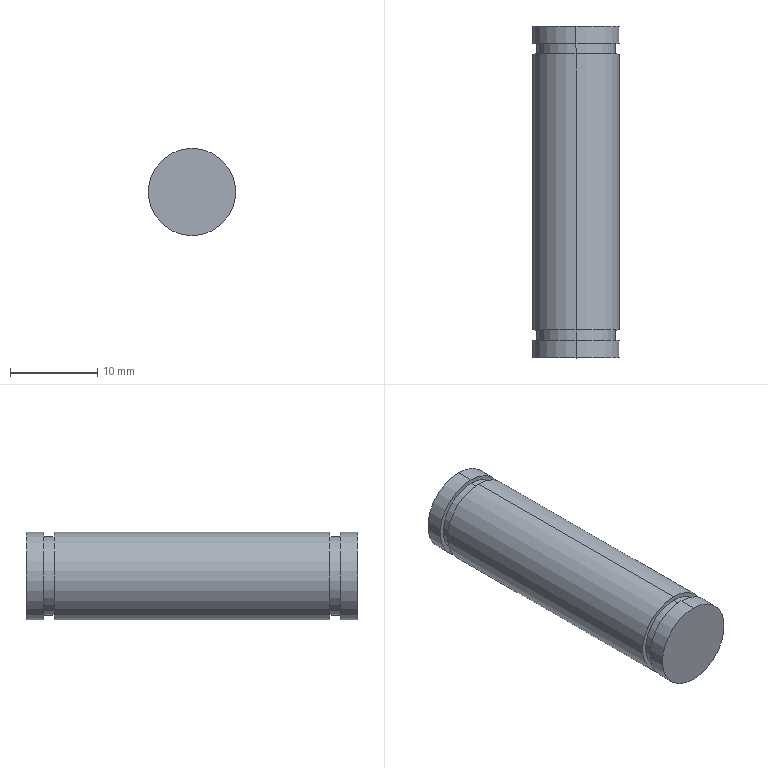Part | SolidWorks | features Revolution 1 | 1 solid | 16 faces | box 10 x 38 x 10 mm | volume 2949 mm3 | cylinder 10 | plane 6 | commonest cylinder face diameters 10 x6 9 x4
STEP:
#1=CARTESIAN_POINT('',(0.,-17.,4.5));
#2=VERTEX_POINT('',#1);
#3=CARTESIAN_POINT('',(0.,-17.,-4.5));
#4=VERTEX_POINT('',#3);
#5=CARTESIAN_POINT('',(0.,-17.,0.));
#6=DIRECTION('',(0.,1.,0.));
#7=DIRECTION('',(0.,0.,1.));
#8=AXIS2_PLACEMENT_3D('',#5,#6,#7);
#9=CIRCLE('',#8,4.5);
#10=EDGE_CURVE('',#2,#4,#9,.T.);
#11=ORIENTED_EDGE('',*,*,#10,.T.);
#12=CARTESIAN_POINT('',(0.,-15.8,-4.5));
#13=VERTEX_POINT('',#12);
#14=CARTESIAN_POINT('',(0.,-19.,-4.5));
#15=DIRECTION('',(0.,1.,0.));
#16=VECTOR('',#15,1000.);
#17=LINE('',#14,#16);
#18=EDGE_CURVE('',#4,#13,#17,.T.);
#19=ORIENTED_EDGE('',*,*,#18,.T.);
#20=CARTESIAN_POINT('',(0.,-15.8,4.5));
#21=VERTEX_POINT('',#20);
#22=CARTESIAN_POINT('',(0.,-15.8,0.));
#23=DIRECTION('',(0.,1.,0.));
#24=DIRECTION('',(0.,0.,1.));
#25=AXIS2_PLACEMENT_3D('',#22,#23,#24);
#26=CIRCLE('',#25,4.5);
#27=EDGE_CURVE('',#21,#13,#26,.T.);
#28=ORIENTED_EDGE('',*,*,#27,.F.);
#29=CARTESIAN_POINT('',(0.,-19.,4.5));
#30=DIRECTION('',(0.,1.,0.));
#31=VECTOR('',#30,1000.);
#32=LINE('',#29,#31);
#33=EDGE_CURVE('',#2,#21,#32,.T.);
#34=ORIENTED_EDGE('',*,*,#33,.F.);
#35=EDGE_LOOP('',(#11,#19,#28,#34));
#36=FACE_OUTER_BOUND('',#35,.T.);
#37=CARTESIAN_POINT('',(0.,-19.,0.));
#38=DIRECTION('',(0.,1.,0.));
#39=DIRECTION('',(0.,0.,1.));
#40=AXIS2_PLACEMENT_3D('',#37,#38,#39);
#41=CYLINDRICAL_SURFACE('',#40,4.5);
#42=ADVANCED_FACE('',(#36),#41,.T.);
#43=CARTESIAN_POINT('',(0.,-15.8,5.));
#44=VERTEX_POINT('',#43);
#45=CARTESIAN_POINT('',(0.,-15.8,-5.));
#46=VERTEX_POINT('',#45);
#47=CARTESIAN_POINT('',(0.,-15.8,0.));
#48=DIRECTION('',(0.,1.,0.));
#49=DIRECTION('',(0.,0.,1.));
#50=AXIS2_PLACEMENT_3D('',#47,#48,#49);
#51=CIRCLE('',#50,5.);
#52=EDGE_CURVE('',#44,#46,#51,.T.);
#53=ORIENTED_EDGE('',*,*,#52,.T.);
#54=CARTESIAN_POINT('',(0.,15.8,-5.));
#55=VERTEX_POINT('',#54);
#56=CARTESIAN_POINT('',(0.,-19.,-5.));
#57=DIRECTION('',(0.,1.,0.));
#58=VECTOR('',#57,1000.);
#59=LINE('',#56,#58);
#60=EDGE_CURVE('',#46,#55,#59,.T.);
#61=ORIENTED_EDGE('',*,*,#60,.T.);
#62=CARTESIAN_POINT('',(0.,15.8,5.));
#63=VERTEX_POINT('',#62);
#64=CARTESIAN_POINT('',(0.,15.8,0.));
#65=DIRECTION('',(0.,1.,0.));
#66=DIRECTION('',(0.,0.,1.));
#67=AXIS2_PLACEMENT_3D('',#64,#65,#66);
#68=CIRCLE('',#67,5.);
#69=EDGE_CURVE('',#63,#55,#68,.T.);
#70=ORIENTED_EDGE('',*,*,#69,.F.);
#71=CARTESIAN_POINT('',(0.,-19.,5.));
#72=DIRECTION('',(0.,1.,0.));
#73=VECTOR('',#72,1000.);
#74=LINE('',#71,#73);
#75=EDGE_CURVE('',#44,#63,#74,.T.);
#76=ORIENTED_EDGE('',*,*,#75,.F.);
#77=EDGE_LOOP('',(#53,#61,#70,#76));
#78=FACE_OUTER_BOUND('',#77,.T.);
#79=CARTESIAN_POINT('',(0.,-19.,0.));
#80=DIRECTION('',(0.,1.,0.));
#81=DIRECTION('',(0.,0.,1.));
#82=AXIS2_PLACEMENT_3D('',#79,#80,#81);
#83=CYLINDRICAL_SURFACE('',#82,5.);
#84=ADVANCED_FACE('',(#78),#83,.T.);
#85=CARTESIAN_POINT('',(0.,15.8,4.5));
#86=VERTEX_POINT('',#85);
#87=CARTESIAN_POINT('',(0.,15.8,-4.5));
#88=VERTEX_POINT('',#87);
#89=CARTESIAN_POINT('',(0.,15.8,0.));
#90=DIRECTION('',(0.,1.,0.));
#91=DIRECTION('',(0.,0.,1.));
#92=AXIS2_PLACEMENT_3D('',#89,#90,#91);
#93=CIRCLE('',#92,4.5);
#94=EDGE_CURVE('',#86,#88,#93,.T.);
#95=ORIENTED_EDGE('',*,*,#94,.T.);
#96=CARTESIAN_POINT('',(0.,17.,-4.5));
#97=VERTEX_POINT('',#96);
#98=CARTESIAN_POINT('',(0.,-19.,-4.5));
#99=DIRECTION('',(0.,1.,0.));
#100=VECTOR('',#99,1000.);
#101=LINE('',#98,#100);
#102=EDGE_CURVE('',#88,#97,#101,.T.);
#103=ORIENTED_EDGE('',*,*,#102,.T.);
#104=CARTESIAN_POINT('',(0.,17.,4.5));
#105=VERTEX_POINT('',#104);
#106=CARTESIAN_POINT('',(0.,17.,0.));
#107=DIRECTION('',(0.,1.,0.));
#108=DIRECTION('',(0.,0.,1.));
#109=AXIS2_PLACEMENT_3D('',#106,#107,#108);
#110=CIRCLE('',#109,4.5);
#111=EDGE_CURVE('',#105,#97,#110,.T.);
#112=ORIENTED_EDGE('',*,*,#111,.F.);
#113=CARTESIAN_POINT('',(0.,-19.,4.5));
#114=DIRECTION('',(0.,1.,0.));
#115=VECTOR('',#114,1000.);
#116=LINE('',#113,#115);
#117=EDGE_CURVE('',#86,#105,#116,.T.);
#118=ORIENTED_EDGE('',*,*,#117,.F.);
#119=EDGE_LOOP('',(#95,#103,#112,#118));
#120=FACE_OUTER_BOUND('',#119,.T.);
#121=CARTESIAN_POINT('',(0.,-19.,0.));
#122=DIRECTION('',(0.,1.,0.));
#123=DIRECTION('',(0.,0.,1.));
#124=AXIS2_PLACEMENT_3D('',#121,#122,#123);
#125=CYLINDRICAL_SURFACE('',#124,4.5);
#126=ADVANCED_FACE('',(#120),#125,.T.);
#127=CARTESIAN_POINT('',(0.,17.,5.));
#128=VERTEX_POINT('',#127);
#129=CARTESIAN_POINT('',(0.,17.,-5.));
#130=VERTEX_POINT('',#129);
#131=CARTESIAN_POINT('',(0.,17.,0.));
#132=DIRECTION('',(0.,1.,0.));
#133=DIRECTION('',(0.,0.,1.));
#134=AXIS2_PLACEMENT_3D('',#131,#132,#133);
#135=CIRCLE('',#134,5.);
#136=EDGE_CURVE('',#128,#130,#135,.T.);
#137=ORIENTED_EDGE('',*,*,#136,.T.);
#138=CARTESIAN_POINT('',(0.,19.,-5.));
#139=VERTEX_POINT('',#138);
#140=CARTESIAN_POINT('',(0.,-19.,-5.));
#141=DIRECTION('',(0.,1.,0.));
#142=VECTOR('',#141,1000.);
#143=LINE('',#140,#142);
#144=EDGE_CURVE('',#130,#139,#143,.T.);
#145=ORIENTED_EDGE('',*,*,#144,.T.);
#146=CARTESIAN_POINT('',(0.,19.,5.));
#147=VERTEX_POINT('',#146);
#148=CARTESIAN_POINT('',(0.,19.,0.));
#149=DIRECTION('',(0.,1.,0.));
#150=DIRECTION('',(0.,0.,1.));
#151=AXIS2_PLACEMENT_3D('',#148,#149,#150);
#152=CIRCLE('',#151,5.);
#153=EDGE_CURVE('',#147,#139,#152,.T.);
#154=ORIENTED_EDGE('',*,*,#153,.F.);
#155=CARTESIAN_POINT('',(0.,-19.,5.));
#156=DIRECTION('',(0.,1.,0.));
#157=VECTOR('',#156,1000.);
#158=LINE('',#155,#157);
#159=EDGE_CURVE('',#128,#147,#158,.T.);
#160=ORIENTED_EDGE('',*,*,#159,.F.);
#161=EDGE_LOOP('',(#137,#145,#154,#160));
#162=FACE_OUTER_BOUND('',#161,.T.);
#163=CARTESIAN_POINT('',(0.,-19.,0.));
#164=DIRECTION('',(0.,1.,0.));
#165=DIRECTION('',(0.,0.,1.));
#166=AXIS2_PLACEMENT_3D('',#163,#164,#165);
#167=CYLINDRICAL_SURFACE('',#166,5.);
#168=ADVANCED_FACE('',(#162),#167,.T.);
#169=CARTESIAN_POINT('',(0.,-19.,5.));
#170=VERTEX_POINT('',#169);
#171=CARTESIAN_POINT('',(0.,-19.,-5.));
#172=VERTEX_POINT('',#171);
#173=CARTESIAN_POINT('',(0.,-19.,0.));
#174=DIRECTION('',(0.,1.,0.));
#175=DIRECTION('',(0.,0.,1.));
#176=AXIS2_PLACEMENT_3D('',#173,#174,#175);
#177=CIRCLE('',#176,5.);
#178=EDGE_CURVE('',#170,#172,#177,.T.);
#179=ORIENTED_EDGE('',*,*,#178,.T.);
#180=CARTESIAN_POINT('',(0.,-17.,-5.));
#181=VERTEX_POINT('',#180);
#182=CARTESIAN_POINT('',(0.,-19.,-5.));
#183=DIRECTION('',(0.,1.,0.));
#184=VECTOR('',#183,1000.);
#185=LINE('',#182,#184);
#186=EDGE_CURVE('',#172,#181,#185,.T.);
#187=ORIENTED_EDGE('',*,*,#186,.T.);
#188=CARTESIAN_POINT('',(0.,-17.,5.));
#189=VERTEX_POINT('',#188);
#190=CARTESIAN_POINT('',(0.,-17.,0.));
#191=DIRECTION('',(0.,1.,0.));
#192=DIRECTION('',(0.,0.,1.));
#193=AXIS2_PLACEMENT_3D('',#190,#191,#192);
#194=CIRCLE('',#193,5.);
#195=EDGE_CURVE('',#189,#181,#194,.T.);
#196=ORIENTED_EDGE('',*,*,#195,.F.);
#197=CARTESIAN_POINT('',(0.,-19.,5.));
#198=DIRECTION('',(0.,1.,0.));
#199=VECTOR('',#198,1000.);
#200=LINE('',#197,#199);
#201=EDGE_CURVE('',#170,#189,#200,.T.);
#202=ORIENTED_EDGE('',*,*,#201,.F.);
#203=EDGE_LOOP('',(#179,#187,#196,#202));
#204=FACE_OUTER_BOUND('',#203,.T.);
#205=CARTESIAN_POINT('',(0.,-19.,0.));
#206=DIRECTION('',(0.,1.,0.));
#207=DIRECTION('',(0.,0.,1.));
#208=AXIS2_PLACEMENT_3D('',#205,#206,#207);
#209=CYLINDRICAL_SURFACE('',#208,5.);
#210=ADVANCED_FACE('',(#204),#209,.T.);
#211=ORIENTED_EDGE('',*,*,#186,.F.);
#212=CARTESIAN_POINT('',(0.,-19.,0.));
#213=DIRECTION('',(0.,1.,0.));
#214=DIRECTION('',(0.,0.,1.));
#215=AXIS2_PLACEMENT_3D('',#212,#213,#214);
#216=CIRCLE('',#215,5.);
#217=EDGE_CURVE('',#172,#170,#216,.T.);
#218=ORIENTED_EDGE('',*,*,#217,.T.);
#219=ORIENTED_EDGE('',*,*,#201,.T.);
#220=CARTESIAN_POINT('',(0.,-17.,0.));
#221=DIRECTION('',(0.,1.,0.));
#222=DIRECTION('',(0.,0.,1.));
#223=AXIS2_PLACEMENT_3D('',#220,#221,#222);
#224=CIRCLE('',#223,5.);
#225=EDGE_CURVE('',#181,#189,#224,.T.);
#226=ORIENTED_EDGE('',*,*,#225,.F.);
#227=EDGE_LOOP('',(#211,#218,#219,#226));
#228=FACE_OUTER_BOUND('',#227,.T.);
#229=CARTESIAN_POINT('',(0.,-19.,0.));
#230=DIRECTION('',(0.,1.,0.));
#231=DIRECTION('',(0.,0.,1.));
#232=AXIS2_PLACEMENT_3D('',#229,#230,#231);
#233=CYLINDRICAL_SURFACE('',#232,5.);
#234=ADVANCED_FACE('',(#228),#233,.T.);
#235=ORIENTED_EDGE('',*,*,#178,.F.);
#236=ORIENTED_EDGE('',*,*,#217,.F.);
#237=EDGE_LOOP('',(#235,#236));
#238=FACE_OUTER_BOUND('',#237,.T.);
#239=CARTESIAN_POINT('',(5.,-19.,0.));
#240=DIRECTION('',(0.,-1.,0.));
#241=DIRECTION('',(0.,0.,-1.));
#242=AXIS2_PLACEMENT_3D('',#239,#240,#241);
#243=PLANE('',#242);
#244=ADVANCED_FACE('',(#238),#243,.T.);
#245=ORIENTED_EDGE('',*,*,#153,.T.);
#246=CARTESIAN_POINT('',(0.,19.,0.));
#247=DIRECTION('',(0.,1.,0.));
#248=DIRECTION('',(0.,0.,1.));
#249=AXIS2_PLACEMENT_3D('',#246,#247,#248);
#250=CIRCLE('',#249,5.);
#251=EDGE_CURVE('',#139,#147,#250,.T.);
#252=ORIENTED_EDGE('',*,*,#251,.T.);
#253=EDGE_LOOP('',(#245,#252));
#254=FACE_OUTER_BOUND('',#253,.T.);
#255=CARTESIAN_POINT('',(0.,19.,0.));
#256=DIRECTION('',(0.,1.,0.));
#257=DIRECTION('',(0.,0.,1.));
#258=AXIS2_PLACEMENT_3D('',#255,#256,#257);
#259=PLANE('',#258);
#260=ADVANCED_FACE('',(#254),#259,.T.);
#261=ORIENTED_EDGE('',*,*,#144,.F.);
#262=CARTESIAN_POINT('',(0.,17.,0.));
#263=DIRECTION('',(0.,1.,0.));
#264=DIRECTION('',(0.,0.,1.));
#265=AXIS2_PLACEMENT_3D('',#262,#263,#264);
#266=CIRCLE('',#265,5.);
#267=EDGE_CURVE('',#130,#128,#266,.T.);
#268=ORIENTED_EDGE('',*,*,#267,.T.);
#269=ORIENTED_EDGE('',*,*,#159,.T.);
#270=ORIENTED_EDGE('',*,*,#251,.F.);
#271=EDGE_LOOP('',(#261,#268,#269,#270));
#272=FACE_OUTER_BOUND('',#271,.T.);
#273=CARTESIAN_POINT('',(0.,-19.,0.));
#274=DIRECTION('',(0.,1.,0.));
#275=DIRECTION('',(0.,0.,1.));
#276=AXIS2_PLACEMENT_3D('',#273,#274,#275);
#277=CYLINDRICAL_SURFACE('',#276,5.);
#278=ADVANCED_FACE('',(#272),#277,.T.);
#279=ORIENTED_EDGE('',*,*,#111,.T.);
#280=CARTESIAN_POINT('',(0.,17.,0.));
#281=DIRECTION('',(0.,1.,0.));
#282=DIRECTION('',(0.,0.,1.));
#283=AXIS2_PLACEMENT_3D('',#280,#281,#282);
#284=CIRCLE('',#283,4.5);
#285=EDGE_CURVE('',#97,#105,#284,.T.);
#286=ORIENTED_EDGE('',*,*,#285,.T.);
#287=EDGE_LOOP('',(#279,#286));
#288=FACE_BOUND('',#287,.T.);
#289=ORIENTED_EDGE('',*,*,#136,.F.);
#290=ORIENTED_EDGE('',*,*,#267,.F.);
#291=EDGE_LOOP('',(#289,#290));
#292=FACE_OUTER_BOUND('',#291,.T.);
#293=CARTESIAN_POINT('',(5.,17.,0.));
#294=DIRECTION('',(0.,-1.,0.));
#295=DIRECTION('',(0.,0.,-1.));
#296=AXIS2_PLACEMENT_3D('',#293,#294,#295);
#297=PLANE('',#296);
#298=ADVANCED_FACE('',(#288,#292),#297,.T.);
#299=ORIENTED_EDGE('',*,*,#102,.F.);
#300=CARTESIAN_POINT('',(0.,15.8,0.));
#301=DIRECTION('',(0.,1.,0.));
#302=DIRECTION('',(0.,0.,1.));
#303=AXIS2_PLACEMENT_3D('',#300,#301,#302);
#304=CIRCLE('',#303,4.5);
#305=EDGE_CURVE('',#88,#86,#304,.T.);
#306=ORIENTED_EDGE('',*,*,#305,.T.);
#307=ORIENTED_EDGE('',*,*,#117,.T.);
#308=ORIENTED_EDGE('',*,*,#285,.F.);
#309=EDGE_LOOP('',(#299,#306,#307,#308));
#310=FACE_OUTER_BOUND('',#309,.T.);
#311=CARTESIAN_POINT('',(0.,-19.,0.));
#312=DIRECTION('',(0.,1.,0.));
#313=DIRECTION('',(0.,0.,1.));
#314=AXIS2_PLACEMENT_3D('',#311,#312,#313);
#315=CYLINDRICAL_SURFACE('',#314,4.5);
#316=ADVANCED_FACE('',(#310),#315,.T.);
#317=ORIENTED_EDGE('',*,*,#69,.T.);
#318=CARTESIAN_POINT('',(0.,15.8,0.));
#319=DIRECTION('',(0.,1.,0.));
#320=DIRECTION('',(0.,0.,1.));
#321=AXIS2_PLACEMENT_3D('',#318,#319,#320);
#322=CIRCLE('',#321,5.);
#323=EDGE_CURVE('',#55,#63,#322,.T.);
#324=ORIENTED_EDGE('',*,*,#323,.T.);
#325=EDGE_LOOP('',(#317,#324));
#326=FACE_OUTER_BOUND('',#325,.T.);
#327=ORIENTED_EDGE('',*,*,#94,.F.);
#328=ORIENTED_EDGE('',*,*,#305,.F.);
#329=EDGE_LOOP('',(#327,#328));
#330=FACE_BOUND('',#329,.T.);
#331=CARTESIAN_POINT('',(4.5,15.8,0.));
#332=DIRECTION('',(0.,1.,0.));
#333=DIRECTION('',(0.,0.,1.));
#334=AXIS2_PLACEMENT_3D('',#331,#332,#333);
#335=PLANE('',#334);
#336=ADVANCED_FACE('',(#326,#330),#335,.T.);
#337=ORIENTED_EDGE('',*,*,#60,.F.);
#338=CARTESIAN_POINT('',(0.,-15.8,0.));
#339=DIRECTION('',(0.,1.,0.));
#340=DIRECTION('',(0.,0.,1.));
#341=AXIS2_PLACEMENT_3D('',#338,#339,#340);
#342=CIRCLE('',#341,5.);
#343=EDGE_CURVE('',#46,#44,#342,.T.);
#344=ORIENTED_EDGE('',*,*,#343,.T.);
#345=ORIENTED_EDGE('',*,*,#75,.T.);
#346=ORIENTED_EDGE('',*,*,#323,.F.);
#347=EDGE_LOOP('',(#337,#344,#345,#346));
#348=FACE_OUTER_BOUND('',#347,.T.);
#349=CARTESIAN_POINT('',(0.,-19.,0.));
#350=DIRECTION('',(0.,1.,0.));
#351=DIRECTION('',(0.,0.,1.));
#352=AXIS2_PLACEMENT_3D('',#349,#350,#351);
#353=CYLINDRICAL_SURFACE('',#352,5.);
#354=ADVANCED_FACE('',(#348),#353,.T.);
#355=ORIENTED_EDGE('',*,*,#27,.T.);
#356=CARTESIAN_POINT('',(0.,-15.8,0.));
#357=DIRECTION('',(0.,1.,0.));
#358=DIRECTION('',(0.,0.,1.));
#359=AXIS2_PLACEMENT_3D('',#356,#357,#358);
#360=CIRCLE('',#359,4.5);
#361=EDGE_CURVE('',#13,#21,#360,.T.);
#362=ORIENTED_EDGE('',*,*,#361,.T.);
#363=EDGE_LOOP('',(#355,#362));
#364=FACE_BOUND('',#363,.T.);
#365=ORIENTED_EDGE('',*,*,#52,.F.);
#366=ORIENTED_EDGE('',*,*,#343,.F.);
#367=EDGE_LOOP('',(#365,#366));
#368=FACE_OUTER_BOUND('',#367,.T.);
#369=CARTESIAN_POINT('',(5.,-15.8,0.));
#370=DIRECTION('',(0.,-1.,0.));
#371=DIRECTION('',(0.,0.,-1.));
#372=AXIS2_PLACEMENT_3D('',#369,#370,#371);
#373=PLANE('',#372);
#374=ADVANCED_FACE('',(#364,#368),#373,.T.);
#375=ORIENTED_EDGE('',*,*,#18,.F.);
#376=CARTESIAN_POINT('',(0.,-17.,0.));
#377=DIRECTION('',(0.,1.,0.));
#378=DIRECTION('',(0.,0.,1.));
#379=AXIS2_PLACEMENT_3D('',#376,#377,#378);
#380=CIRCLE('',#379,4.5);
#381=EDGE_CURVE('',#4,#2,#380,.T.);
#382=ORIENTED_EDGE('',*,*,#381,.T.);
#383=ORIENTED_EDGE('',*,*,#33,.T.);
#384=ORIENTED_EDGE('',*,*,#361,.F.);
#385=EDGE_LOOP('',(#375,#382,#383,#384));
#386=FACE_OUTER_BOUND('',#385,.T.);
#387=CARTESIAN_POINT('',(0.,-19.,0.));
#388=DIRECTION('',(0.,1.,0.));
#389=DIRECTION('',(0.,0.,1.));
#390=AXIS2_PLACEMENT_3D('',#387,#388,#389);
#391=CYLINDRICAL_SURFACE('',#390,4.5);
#392=ADVANCED_FACE('',(#386),#391,.T.);
#393=ORIENTED_EDGE('',*,*,#195,.T.);
#394=ORIENTED_EDGE('',*,*,#225,.T.);
#395=EDGE_LOOP('',(#393,#394));
#396=FACE_OUTER_BOUND('',#395,.T.);
#397=ORIENTED_EDGE('',*,*,#10,.F.);
#398=ORIENTED_EDGE('',*,*,#381,.F.);
#399=EDGE_LOOP('',(#397,#398));
#400=FACE_BOUND('',#399,.T.);
#401=CARTESIAN_POINT('',(4.5,-17.,0.));
#402=DIRECTION('',(0.,1.,0.));
#403=DIRECTION('',(0.,0.,1.));
#404=AXIS2_PLACEMENT_3D('',#401,#402,#403);
#405=PLANE('',#404);
#406=ADVANCED_FACE('',(#396,#400),#405,.T.);
#407=CLOSED_SHELL('',(#42,#84,#126,#168,#210,#234,#244,#260,#278,#298,#316,#336,#354,#374,#392,#406));
#408=MANIFOLD_SOLID_BREP('',#407);
#409=CARTESIAN_POINT('',(0.,0.,0.));
#410=DIRECTION('',(0.,0.,1.));
#411=DIRECTION('',(1.,0.,0.));
#412=AXIS2_PLACEMENT_3D('',#409,#410,#411);
#413=(LENGTH_UNIT()NAMED_UNIT(*)SI_UNIT(.MILLI.,.METRE.));
#414=UNCERTAINTY_MEASURE_WITH_UNIT(LENGTH_MEASURE(0.00001),#413,'','');
#415=(NAMED_UNIT(*)PLANE_ANGLE_UNIT()SI_UNIT($,.RADIAN.));
#416=(NAMED_UNIT(*)SI_UNIT($,.STERADIAN.)SOLID_ANGLE_UNIT());
#417=(GEOMETRIC_REPRESENTATION_CONTEXT(3)GLOBAL_UNCERTAINTY_ASSIGNED_CONTEXT((#414))GLOBAL_UNIT_ASSIGNED_CONTEXT((#413,#415,#416))REPRESENTATION_CONTEXT('',''));
#418=ADVANCED_BREP_SHAPE_REPRESENTATION('',(#408,#412),#417);